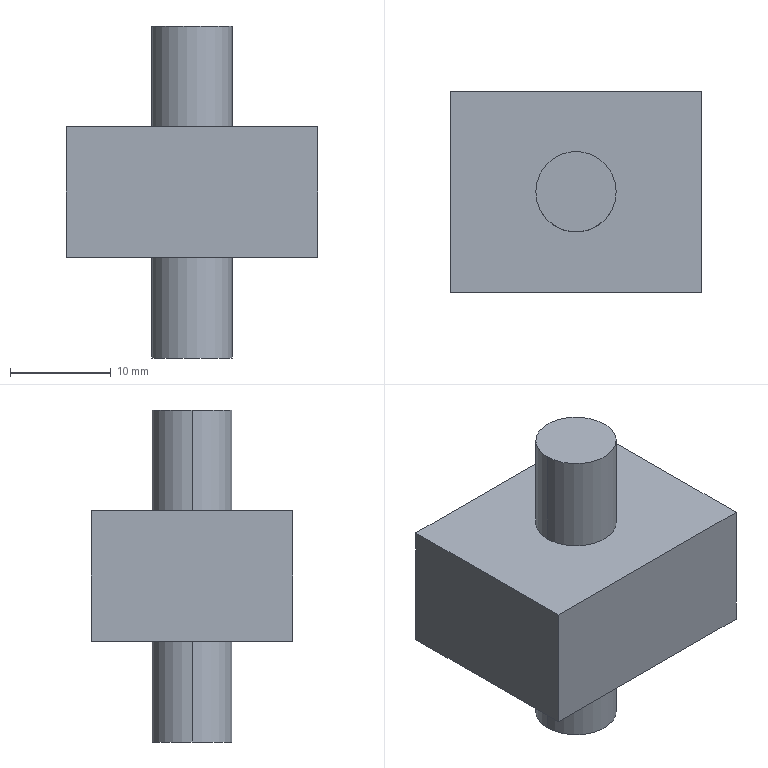Part | SolidWorks | features Extrusion 1, ICE 1, MirrorPattern 1 | 1 solid | 12 faces | box 25 x 20 x 33 mm | volume 7505 mm3 | plane 8 | cylinder 4 | commonest cylinder face diameters 8 x4
STEP:
#1=CARTESIAN_POINT('',(4.,10.,-16.5));
#2=VERTEX_POINT('',#1);
#3=CARTESIAN_POINT('',(-4.,10.,-16.5));
#4=VERTEX_POINT('',#3);
#5=CARTESIAN_POINT('',(0.,10.,-16.5));
#6=DIRECTION('',(0.,0.,1.));
#7=DIRECTION('',(1.,0.,0.));
#8=AXIS2_PLACEMENT_3D('',#5,#6,#7);
#9=CIRCLE('',#8,4.);
#10=EDGE_CURVE('',#2,#4,#9,.T.);
#11=ORIENTED_EDGE('',*,*,#10,.T.);
#12=CARTESIAN_POINT('',(-4.,10.,-6.5));
#13=VERTEX_POINT('',#12);
#14=CARTESIAN_POINT('',(-4.,10.,-16.5));
#15=DIRECTION('',(0.,0.,1.));
#16=VECTOR('',#15,1000.);
#17=LINE('',#14,#16);
#18=EDGE_CURVE('',#4,#13,#17,.T.);
#19=ORIENTED_EDGE('',*,*,#18,.T.);
#20=CARTESIAN_POINT('',(4.,10.,-6.5));
#21=VERTEX_POINT('',#20);
#22=CARTESIAN_POINT('',(0.,10.,-6.5));
#23=DIRECTION('',(0.,0.,1.));
#24=DIRECTION('',(1.,0.,0.));
#25=AXIS2_PLACEMENT_3D('',#22,#23,#24);
#26=CIRCLE('',#25,4.);
#27=EDGE_CURVE('',#21,#13,#26,.T.);
#28=ORIENTED_EDGE('',*,*,#27,.F.);
#29=CARTESIAN_POINT('',(4.,10.,-16.5));
#30=DIRECTION('',(0.,0.,1.));
#31=VECTOR('',#30,1000.);
#32=LINE('',#29,#31);
#33=EDGE_CURVE('',#2,#21,#32,.T.);
#34=ORIENTED_EDGE('',*,*,#33,.F.);
#35=EDGE_LOOP('',(#11,#19,#28,#34));
#36=FACE_OUTER_BOUND('',#35,.T.);
#37=CARTESIAN_POINT('',(0.,10.,-16.5));
#38=DIRECTION('',(0.,0.,1.));
#39=DIRECTION('',(1.,0.,0.));
#40=AXIS2_PLACEMENT_3D('',#37,#38,#39);
#41=CYLINDRICAL_SURFACE('',#40,4.);
#42=ADVANCED_FACE('',(#36),#41,.T.);
#43=CARTESIAN_POINT('',(4.,10.,16.5));
#44=VERTEX_POINT('',#43);
#45=CARTESIAN_POINT('',(-4.,10.,16.5));
#46=VERTEX_POINT('',#45);
#47=CARTESIAN_POINT('',(0.,10.,16.5));
#48=DIRECTION('',(0.,0.,1.));
#49=DIRECTION('',(1.,0.,0.));
#50=AXIS2_PLACEMENT_3D('',#47,#48,#49);
#51=CIRCLE('',#50,4.);
#52=EDGE_CURVE('',#44,#46,#51,.T.);
#53=ORIENTED_EDGE('',*,*,#52,.F.);
#54=CARTESIAN_POINT('',(4.,10.,6.5));
#55=VERTEX_POINT('',#54);
#56=CARTESIAN_POINT('',(4.,10.,16.5));
#57=DIRECTION('',(0.,0.,-1.));
#58=VECTOR('',#57,1000.);
#59=LINE('',#56,#58);
#60=EDGE_CURVE('',#44,#55,#59,.T.);
#61=ORIENTED_EDGE('',*,*,#60,.T.);
#62=CARTESIAN_POINT('',(-4.,10.,6.5));
#63=VERTEX_POINT('',#62);
#64=CARTESIAN_POINT('',(0.,10.,6.5));
#65=DIRECTION('',(0.,0.,1.));
#66=DIRECTION('',(1.,0.,0.));
#67=AXIS2_PLACEMENT_3D('',#64,#65,#66);
#68=CIRCLE('',#67,4.);
#69=EDGE_CURVE('',#55,#63,#68,.T.);
#70=ORIENTED_EDGE('',*,*,#69,.T.);
#71=CARTESIAN_POINT('',(-4.,10.,16.5));
#72=DIRECTION('',(0.,0.,-1.));
#73=VECTOR('',#72,1000.);
#74=LINE('',#71,#73);
#75=EDGE_CURVE('',#46,#63,#74,.T.);
#76=ORIENTED_EDGE('',*,*,#75,.F.);
#77=EDGE_LOOP('',(#53,#61,#70,#76));
#78=FACE_OUTER_BOUND('',#77,.T.);
#79=CARTESIAN_POINT('',(0.,10.,16.5));
#80=DIRECTION('',(0.,0.,-1.));
#81=DIRECTION('',(-1.,0.,0.));
#82=AXIS2_PLACEMENT_3D('',#79,#80,#81);
#83=CYLINDRICAL_SURFACE('',#82,4.);
#84=ADVANCED_FACE('',(#78),#83,.T.);
#85=CARTESIAN_POINT('',(12.5,0.,6.5));
#86=VERTEX_POINT('',#85);
#87=CARTESIAN_POINT('',(12.5,0.,-6.5));
#88=VERTEX_POINT('',#87);
#89=CARTESIAN_POINT('',(12.5,0.,6.5));
#90=DIRECTION('',(0.,0.,-1.));
#91=VECTOR('',#90,1000.);
#92=LINE('',#89,#91);
#93=EDGE_CURVE('',#86,#88,#92,.T.);
#94=ORIENTED_EDGE('',*,*,#93,.T.);
#95=CARTESIAN_POINT('',(12.5,20.,-6.5));
#96=VERTEX_POINT('',#95);
#97=CARTESIAN_POINT('',(12.5,20.,-6.5));
#98=DIRECTION('',(0.,-1.,0.));
#99=VECTOR('',#98,1000.);
#100=LINE('',#97,#99);
#101=EDGE_CURVE('',#96,#88,#100,.T.);
#102=ORIENTED_EDGE('',*,*,#101,.F.);
#103=CARTESIAN_POINT('',(12.5,20.,6.5));
#104=VERTEX_POINT('',#103);
#105=CARTESIAN_POINT('',(12.5,20.,6.5));
#106=DIRECTION('',(0.,0.,-1.));
#107=VECTOR('',#106,1000.);
#108=LINE('',#105,#107);
#109=EDGE_CURVE('',#104,#96,#108,.T.);
#110=ORIENTED_EDGE('',*,*,#109,.F.);
#111=CARTESIAN_POINT('',(12.5,20.,6.5));
#112=DIRECTION('',(0.,-1.,0.));
#113=VECTOR('',#112,1000.);
#114=LINE('',#111,#113);
#115=EDGE_CURVE('',#104,#86,#114,.T.);
#116=ORIENTED_EDGE('',*,*,#115,.T.);
#117=EDGE_LOOP('',(#94,#102,#110,#116));
#118=FACE_OUTER_BOUND('',#117,.T.);
#119=CARTESIAN_POINT('',(12.5,20.,6.5));
#120=DIRECTION('',(-1.,0.,0.));
#121=DIRECTION('',(0.,0.,1.));
#122=AXIS2_PLACEMENT_3D('',#119,#120,#121);
#123=PLANE('',#122);
#124=ADVANCED_FACE('',(#118),#123,.F.);
#125=ORIENTED_EDGE('',*,*,#27,.T.);
#126=CARTESIAN_POINT('',(0.,10.,-6.5));
#127=DIRECTION('',(0.,0.,1.));
#128=DIRECTION('',(1.,0.,0.));
#129=AXIS2_PLACEMENT_3D('',#126,#127,#128);
#130=CIRCLE('',#129,4.);
#131=EDGE_CURVE('',#13,#21,#130,.T.);
#132=ORIENTED_EDGE('',*,*,#131,.T.);
#133=EDGE_LOOP('',(#125,#132));
#134=FACE_BOUND('',#133,.T.);
#135=CARTESIAN_POINT('',(-12.5,0.,-6.5));
#136=VERTEX_POINT('',#135);
#137=CARTESIAN_POINT('',(-12.5,0.,-6.5));
#138=DIRECTION('',(-1.,0.,0.));
#139=VECTOR('',#138,1000.);
#140=LINE('',#137,#139);
#141=EDGE_CURVE('',#88,#136,#140,.T.);
#142=ORIENTED_EDGE('',*,*,#141,.T.);
#143=CARTESIAN_POINT('',(-12.5,20.,-6.5));
#144=VERTEX_POINT('',#143);
#145=CARTESIAN_POINT('',(-12.5,20.,-6.5));
#146=DIRECTION('',(0.,-1.,0.));
#147=VECTOR('',#146,1000.);
#148=LINE('',#145,#147);
#149=EDGE_CURVE('',#144,#136,#148,.T.);
#150=ORIENTED_EDGE('',*,*,#149,.F.);
#151=CARTESIAN_POINT('',(-12.5,20.,-6.5));
#152=DIRECTION('',(-1.,0.,0.));
#153=VECTOR('',#152,1000.);
#154=LINE('',#151,#153);
#155=EDGE_CURVE('',#96,#144,#154,.T.);
#156=ORIENTED_EDGE('',*,*,#155,.F.);
#157=ORIENTED_EDGE('',*,*,#101,.T.);
#158=EDGE_LOOP('',(#142,#150,#156,#157));
#159=FACE_OUTER_BOUND('',#158,.T.);
#160=CARTESIAN_POINT('',(-12.5,20.,-6.5));
#161=DIRECTION('',(0.,0.,1.));
#162=DIRECTION('',(1.,0.,0.));
#163=AXIS2_PLACEMENT_3D('',#160,#161,#162);
#164=PLANE('',#163);
#165=ADVANCED_FACE('',(#134,#159),#164,.F.);
#166=CARTESIAN_POINT('',(-12.5,0.,6.5));
#167=VERTEX_POINT('',#166);
#168=CARTESIAN_POINT('',(-12.5,0.,6.5));
#169=DIRECTION('',(0.,0.,1.));
#170=VECTOR('',#169,1000.);
#171=LINE('',#168,#170);
#172=EDGE_CURVE('',#136,#167,#171,.T.);
#173=ORIENTED_EDGE('',*,*,#172,.T.);
#174=CARTESIAN_POINT('',(-12.5,20.,6.5));
#175=VERTEX_POINT('',#174);
#176=CARTESIAN_POINT('',(-12.5,20.,6.5));
#177=DIRECTION('',(0.,-1.,0.));
#178=VECTOR('',#177,1000.);
#179=LINE('',#176,#178);
#180=EDGE_CURVE('',#175,#167,#179,.T.);
#181=ORIENTED_EDGE('',*,*,#180,.F.);
#182=CARTESIAN_POINT('',(-12.5,20.,6.5));
#183=DIRECTION('',(0.,0.,1.));
#184=VECTOR('',#183,1000.);
#185=LINE('',#182,#184);
#186=EDGE_CURVE('',#144,#175,#185,.T.);
#187=ORIENTED_EDGE('',*,*,#186,.F.);
#188=ORIENTED_EDGE('',*,*,#149,.T.);
#189=EDGE_LOOP('',(#173,#181,#187,#188));
#190=FACE_OUTER_BOUND('',#189,.T.);
#191=CARTESIAN_POINT('',(-12.5,20.,6.5));
#192=DIRECTION('',(1.,0.,0.));
#193=DIRECTION('',(0.,0.,-1.));
#194=AXIS2_PLACEMENT_3D('',#191,#192,#193);
#195=PLANE('',#194);
#196=ADVANCED_FACE('',(#190),#195,.F.);
#197=CARTESIAN_POINT('',(0.,10.,6.5));
#198=DIRECTION('',(0.,0.,1.));
#199=DIRECTION('',(1.,0.,0.));
#200=AXIS2_PLACEMENT_3D('',#197,#198,#199);
#201=CIRCLE('',#200,4.);
#202=EDGE_CURVE('',#63,#55,#201,.T.);
#203=ORIENTED_EDGE('',*,*,#202,.F.);
#204=ORIENTED_EDGE('',*,*,#69,.F.);
#205=EDGE_LOOP('',(#203,#204));
#206=FACE_BOUND('',#205,.T.);
#207=CARTESIAN_POINT('',(-12.5,0.,6.5));
#208=DIRECTION('',(1.,0.,0.));
#209=VECTOR('',#208,1000.);
#210=LINE('',#207,#209);
#211=EDGE_CURVE('',#167,#86,#210,.T.);
#212=ORIENTED_EDGE('',*,*,#211,.T.);
#213=ORIENTED_EDGE('',*,*,#115,.F.);
#214=CARTESIAN_POINT('',(-12.5,20.,6.5));
#215=DIRECTION('',(1.,0.,0.));
#216=VECTOR('',#215,1000.);
#217=LINE('',#214,#216);
#218=EDGE_CURVE('',#175,#104,#217,.T.);
#219=ORIENTED_EDGE('',*,*,#218,.F.);
#220=ORIENTED_EDGE('',*,*,#180,.T.);
#221=EDGE_LOOP('',(#212,#213,#219,#220));
#222=FACE_OUTER_BOUND('',#221,.T.);
#223=CARTESIAN_POINT('',(-12.5,20.,6.5));
#224=DIRECTION('',(0.,0.,-1.));
#225=DIRECTION('',(-1.,0.,0.));
#226=AXIS2_PLACEMENT_3D('',#223,#224,#225);
#227=PLANE('',#226);
#228=ADVANCED_FACE('',(#206,#222),#227,.F.);
#229=ORIENTED_EDGE('',*,*,#109,.T.);
#230=ORIENTED_EDGE('',*,*,#155,.T.);
#231=ORIENTED_EDGE('',*,*,#186,.T.);
#232=ORIENTED_EDGE('',*,*,#218,.T.);
#233=EDGE_LOOP('',(#229,#230,#231,#232));
#234=FACE_OUTER_BOUND('',#233,.T.);
#235=CARTESIAN_POINT('',(0.,20.,0.));
#236=DIRECTION('',(0.,-1.,0.));
#237=DIRECTION('',(0.,0.,-1.));
#238=AXIS2_PLACEMENT_3D('',#235,#236,#237);
#239=PLANE('',#238);
#240=ADVANCED_FACE('',(#234),#239,.F.);
#241=ORIENTED_EDGE('',*,*,#93,.F.);
#242=ORIENTED_EDGE('',*,*,#211,.F.);
#243=ORIENTED_EDGE('',*,*,#172,.F.);
#244=ORIENTED_EDGE('',*,*,#141,.F.);
#245=EDGE_LOOP('',(#241,#242,#243,#244));
#246=FACE_OUTER_BOUND('',#245,.T.);
#247=CARTESIAN_POINT('',(0.,0.,0.));
#248=DIRECTION('',(0.,-1.,0.));
#249=DIRECTION('',(0.,0.,-1.));
#250=AXIS2_PLACEMENT_3D('',#247,#248,#249);
#251=PLANE('',#250);
#252=ADVANCED_FACE('',(#246),#251,.T.);
#253=ORIENTED_EDGE('',*,*,#60,.F.);
#254=CARTESIAN_POINT('',(0.,10.,16.5));
#255=DIRECTION('',(0.,0.,1.));
#256=DIRECTION('',(1.,0.,0.));
#257=AXIS2_PLACEMENT_3D('',#254,#255,#256);
#258=CIRCLE('',#257,4.);
#259=EDGE_CURVE('',#46,#44,#258,.T.);
#260=ORIENTED_EDGE('',*,*,#259,.F.);
#261=ORIENTED_EDGE('',*,*,#75,.T.);
#262=ORIENTED_EDGE('',*,*,#202,.T.);
#263=EDGE_LOOP('',(#253,#260,#261,#262));
#264=FACE_OUTER_BOUND('',#263,.T.);
#265=CARTESIAN_POINT('',(0.,10.,16.5));
#266=DIRECTION('',(0.,0.,-1.));
#267=DIRECTION('',(-1.,0.,0.));
#268=AXIS2_PLACEMENT_3D('',#265,#266,#267);
#269=CYLINDRICAL_SURFACE('',#268,4.);
#270=ADVANCED_FACE('',(#264),#269,.T.);
#271=ORIENTED_EDGE('',*,*,#259,.T.);
#272=ORIENTED_EDGE('',*,*,#52,.T.);
#273=EDGE_LOOP('',(#271,#272));
#274=FACE_OUTER_BOUND('',#273,.T.);
#275=CARTESIAN_POINT('',(0.,10.,16.5));
#276=DIRECTION('',(0.,0.,1.));
#277=DIRECTION('',(1.,0.,0.));
#278=AXIS2_PLACEMENT_3D('',#275,#276,#277);
#279=PLANE('',#278);
#280=ADVANCED_FACE('',(#274),#279,.T.);
#281=ORIENTED_EDGE('',*,*,#18,.F.);
#282=CARTESIAN_POINT('',(0.,10.,-16.5));
#283=DIRECTION('',(0.,0.,1.));
#284=DIRECTION('',(1.,0.,0.));
#285=AXIS2_PLACEMENT_3D('',#282,#283,#284);
#286=CIRCLE('',#285,4.);
#287=EDGE_CURVE('',#4,#2,#286,.T.);
#288=ORIENTED_EDGE('',*,*,#287,.T.);
#289=ORIENTED_EDGE('',*,*,#33,.T.);
#290=ORIENTED_EDGE('',*,*,#131,.F.);
#291=EDGE_LOOP('',(#281,#288,#289,#290));
#292=FACE_OUTER_BOUND('',#291,.T.);
#293=CARTESIAN_POINT('',(0.,10.,-16.5));
#294=DIRECTION('',(0.,0.,1.));
#295=DIRECTION('',(1.,0.,0.));
#296=AXIS2_PLACEMENT_3D('',#293,#294,#295);
#297=CYLINDRICAL_SURFACE('',#296,4.);
#298=ADVANCED_FACE('',(#292),#297,.T.);
#299=ORIENTED_EDGE('',*,*,#10,.F.);
#300=ORIENTED_EDGE('',*,*,#287,.F.);
#301=EDGE_LOOP('',(#299,#300));
#302=FACE_OUTER_BOUND('',#301,.T.);
#303=CARTESIAN_POINT('',(0.,10.,-16.5));
#304=DIRECTION('',(0.,0.,-1.));
#305=DIRECTION('',(1.,0.,0.));
#306=AXIS2_PLACEMENT_3D('',#303,#304,#305);
#307=PLANE('',#306);
#308=ADVANCED_FACE('',(#302),#307,.T.);
#309=CLOSED_SHELL('',(#42,#84,#124,#165,#196,#228,#240,#252,#270,#280,#298,#308));
#310=MANIFOLD_SOLID_BREP('',#309);
#311=CARTESIAN_POINT('',(0.,0.,0.));
#312=DIRECTION('',(0.,0.,1.));
#313=DIRECTION('',(1.,0.,0.));
#314=AXIS2_PLACEMENT_3D('',#311,#312,#313);
#315=(LENGTH_UNIT()NAMED_UNIT(*)SI_UNIT(.MILLI.,.METRE.));
#316=UNCERTAINTY_MEASURE_WITH_UNIT(LENGTH_MEASURE(0.00001),#315,'','');
#317=(NAMED_UNIT(*)PLANE_ANGLE_UNIT()SI_UNIT($,.RADIAN.));
#318=(NAMED_UNIT(*)SI_UNIT($,.STERADIAN.)SOLID_ANGLE_UNIT());
#319=(GEOMETRIC_REPRESENTATION_CONTEXT(3)GLOBAL_UNCERTAINTY_ASSIGNED_CONTEXT((#316))GLOBAL_UNIT_ASSIGNED_CONTEXT((#315,#317,#318))REPRESENTATION_CONTEXT('',''));
#320=ADVANCED_BREP_SHAPE_REPRESENTATION('',(#310,#314),#319);